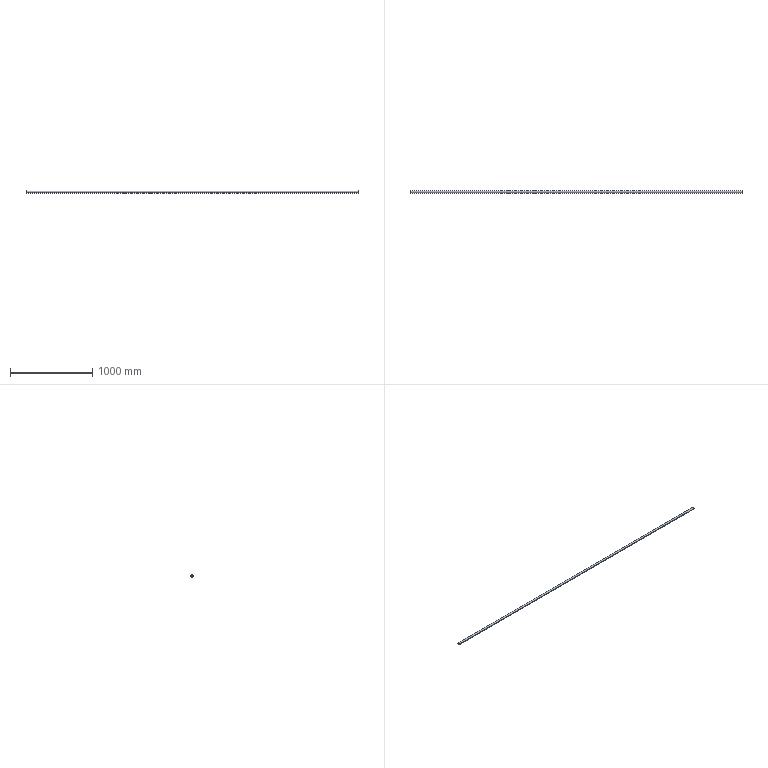Part | STEP file | 电柜护栏1栏杆_Default<As Machined> | 1 solid | 6 faces | box 4025 x 25 x 25 mm | volume 445733 mm3 | cylinder 4 | plane 2 | commonest cylinder face diameters 22 x2 25 x2
STEP:
#1=CARTESIAN_POINT('',(0.,0.,0.));
#2=DIRECTION('',(0.,0.,1.));
#3=DIRECTION('',(1.,0.,0.));
#4=AXIS2_PLACEMENT_3D('',#1,#2,#3);
#5=CARTESIAN_POINT('',(2012.5,12.5,0.));
#6=VERTEX_POINT('',#5);
#7=CARTESIAN_POINT('',(2012.5,-12.5,0.));
#8=VERTEX_POINT('',#7);
#9=CARTESIAN_POINT('',(2012.5,0.,0.));
#10=DIRECTION('',(1.,0.,0.));
#11=DIRECTION('',(0.,1.,0.));
#12=AXIS2_PLACEMENT_3D('',#9,#10,#11);
#13=CIRCLE('',#12,12.5);
#14=CARTESIAN_POINT('',(2012.5,0.,0.));
#15=DIRECTION('',(-1.,0.,0.));
#16=DIRECTION('',(0.,-1.,0.));
#17=AXIS2_PLACEMENT_3D('',#14,#15,#16);
#18=CYLINDRICAL_SURFACE('',#17,12.5);
#19=CARTESIAN_POINT('',(3.142,0.));
#20=DIRECTION('',(-1.,0.));
#21=VECTOR('',#20,1.);
#22=LINE('',#19,#21);
#23=(GEOMETRIC_REPRESENTATION_CONTEXT(2)PARAMETRIC_REPRESENTATION_CONTEXT()REPRESENTATION_CONTEXT('',''));
#24=DEFINITIONAL_REPRESENTATION('',(#22),#23);
#25=PCURVE('',#18,#24);
#26=CARTESIAN_POINT('',(2012.5,0.,0.));
#27=DIRECTION('',(1.,0.,0.));
#28=DIRECTION('',(0.,1.,0.));
#29=AXIS2_PLACEMENT_3D('',#26,#27,#28);
#30=PLANE('',#29);
#31=CARTESIAN_POINT('',(0.,0.));
#32=DIRECTION('',(1.,0.));
#33=AXIS2_PLACEMENT_2D('',#31,#32);
#34=CIRCLE('',#33,12.5);
#35=(GEOMETRIC_REPRESENTATION_CONTEXT(2)PARAMETRIC_REPRESENTATION_CONTEXT()REPRESENTATION_CONTEXT('',''));
#36=DEFINITIONAL_REPRESENTATION('',(#34),#35);
#37=PCURVE('',#30,#36);
#38=SURFACE_CURVE('',#13,(#25,#37),.PCURVE_S1.);
#39=EDGE_CURVE('',#6,#8,#38,.T.);
#40=ORIENTED_EDGE('',*,*,#39,.F.);
#41=CARTESIAN_POINT('',(-2012.5,12.5,0.));
#42=VERTEX_POINT('',#41);
#43=CARTESIAN_POINT('',(2012.5,12.5,0.));
#44=DIRECTION('',(-1.,0.,0.));
#45=VECTOR('',#44,1.);
#46=LINE('',#43,#45);
#47=CARTESIAN_POINT('',(3.142,0.));
#48=DIRECTION('',(0.,1.));
#49=VECTOR('',#48,1.);
#50=LINE('',#47,#49);
#51=(GEOMETRIC_REPRESENTATION_CONTEXT(2)PARAMETRIC_REPRESENTATION_CONTEXT()REPRESENTATION_CONTEXT('',''));
#52=DEFINITIONAL_REPRESENTATION('',(#50),#51);
#53=PCURVE('',#18,#52);
#54=CARTESIAN_POINT('',(2012.5,0.,0.));
#55=DIRECTION('',(-1.,0.,0.));
#56=DIRECTION('',(0.,-1.,0.));
#57=AXIS2_PLACEMENT_3D('',#54,#55,#56);
#58=CYLINDRICAL_SURFACE('',#57,12.5);
#59=CARTESIAN_POINT('',(3.142,0.));
#60=DIRECTION('',(0.,1.));
#61=VECTOR('',#60,1.);
#62=LINE('',#59,#61);
#63=(GEOMETRIC_REPRESENTATION_CONTEXT(2)PARAMETRIC_REPRESENTATION_CONTEXT()REPRESENTATION_CONTEXT('',''));
#64=DEFINITIONAL_REPRESENTATION('',(#62),#63);
#65=PCURVE('',#58,#64);
#66=SURFACE_CURVE('',#46,(#53,#65),.PCURVE_S1.);
#67=EDGE_CURVE('',#6,#42,#66,.T.);
#68=ORIENTED_EDGE('',*,*,#67,.T.);
#69=CARTESIAN_POINT('',(-2012.5,-12.5,0.));
#70=VERTEX_POINT('',#69);
#71=CARTESIAN_POINT('',(-2012.5,0.,0.));
#72=DIRECTION('',(1.,0.,0.));
#73=DIRECTION('',(0.,1.,0.));
#74=AXIS2_PLACEMENT_3D('',#71,#72,#73);
#75=CIRCLE('',#74,12.5);
#76=CARTESIAN_POINT('',(3.142,4025.));
#77=DIRECTION('',(-1.,0.));
#78=VECTOR('',#77,1.);
#79=LINE('',#76,#78);
#80=(GEOMETRIC_REPRESENTATION_CONTEXT(2)PARAMETRIC_REPRESENTATION_CONTEXT()REPRESENTATION_CONTEXT('',''));
#81=DEFINITIONAL_REPRESENTATION('',(#79),#80);
#82=PCURVE('',#18,#81);
#83=CARTESIAN_POINT('',(-2012.5,0.,0.));
#84=DIRECTION('',(1.,0.,0.));
#85=DIRECTION('',(0.,1.,0.));
#86=AXIS2_PLACEMENT_3D('',#83,#84,#85);
#87=PLANE('',#86);
#88=CARTESIAN_POINT('',(0.,0.));
#89=DIRECTION('',(1.,0.));
#90=AXIS2_PLACEMENT_2D('',#88,#89);
#91=CIRCLE('',#90,12.5);
#92=(GEOMETRIC_REPRESENTATION_CONTEXT(2)PARAMETRIC_REPRESENTATION_CONTEXT()REPRESENTATION_CONTEXT('',''));
#93=DEFINITIONAL_REPRESENTATION('',(#91),#92);
#94=PCURVE('',#87,#93);
#95=SURFACE_CURVE('',#75,(#82,#94),.PCURVE_S1.);
#96=EDGE_CURVE('',#42,#70,#95,.T.);
#97=ORIENTED_EDGE('',*,*,#96,.T.);
#98=CARTESIAN_POINT('',(2012.5,-12.5,0.));
#99=DIRECTION('',(-1.,0.,0.));
#100=VECTOR('',#99,1.);
#101=LINE('',#98,#100);
#102=CARTESIAN_POINT('',(0.,0.));
#103=DIRECTION('',(0.,1.));
#104=VECTOR('',#103,1.);
#105=LINE('',#102,#104);
#106=(GEOMETRIC_REPRESENTATION_CONTEXT(2)PARAMETRIC_REPRESENTATION_CONTEXT()REPRESENTATION_CONTEXT('',''));
#107=DEFINITIONAL_REPRESENTATION('',(#105),#106);
#108=PCURVE('',#18,#107);
#109=CARTESIAN_POINT('',(6.283,0.));
#110=DIRECTION('',(0.,1.));
#111=VECTOR('',#110,1.);
#112=LINE('',#109,#111);
#113=(GEOMETRIC_REPRESENTATION_CONTEXT(2)PARAMETRIC_REPRESENTATION_CONTEXT()REPRESENTATION_CONTEXT('',''));
#114=DEFINITIONAL_REPRESENTATION('',(#112),#113);
#115=PCURVE('',#58,#114);
#116=SURFACE_CURVE('',#101,(#108,#115),.PCURVE_S1.);
#117=EDGE_CURVE('',#8,#70,#116,.T.);
#118=ORIENTED_EDGE('',*,*,#117,.F.);
#119=EDGE_LOOP('',(#40,#68,#97,#118));
#120=FACE_BOUND('',#119,.T.);
#121=ADVANCED_FACE('',(#120),#18,.T.);
#122=CARTESIAN_POINT('',(2012.5,-11.,0.));
#123=VERTEX_POINT('',#122);
#124=CARTESIAN_POINT('',(-2012.5,-11.,0.));
#125=VERTEX_POINT('',#124);
#126=CARTESIAN_POINT('',(2012.5,-11.,0.));
#127=DIRECTION('',(-1.,0.,0.));
#128=VECTOR('',#127,1.);
#129=LINE('',#126,#128);
#130=CARTESIAN_POINT('',(2012.5,0.,0.));
#131=DIRECTION('',(-1.,0.,0.));
#132=DIRECTION('',(0.,-1.,0.));
#133=AXIS2_PLACEMENT_3D('',#130,#131,#132);
#134=CYLINDRICAL_SURFACE('',#133,11.);
#135=CARTESIAN_POINT('',(6.283,0.));
#136=DIRECTION('',(0.,1.));
#137=VECTOR('',#136,1.);
#138=LINE('',#135,#137);
#139=(GEOMETRIC_REPRESENTATION_CONTEXT(2)PARAMETRIC_REPRESENTATION_CONTEXT()REPRESENTATION_CONTEXT('',''));
#140=DEFINITIONAL_REPRESENTATION('',(#138),#139);
#141=PCURVE('',#134,#140);
#142=CARTESIAN_POINT('',(2012.5,0.,0.));
#143=DIRECTION('',(-1.,0.,0.));
#144=DIRECTION('',(0.,-1.,0.));
#145=AXIS2_PLACEMENT_3D('',#142,#143,#144);
#146=CYLINDRICAL_SURFACE('',#145,11.);
#147=CARTESIAN_POINT('',(0.,0.));
#148=DIRECTION('',(0.,1.));
#149=VECTOR('',#148,1.);
#150=LINE('',#147,#149);
#151=(GEOMETRIC_REPRESENTATION_CONTEXT(2)PARAMETRIC_REPRESENTATION_CONTEXT()REPRESENTATION_CONTEXT('',''));
#152=DEFINITIONAL_REPRESENTATION('',(#150),#151);
#153=PCURVE('',#146,#152);
#154=SURFACE_CURVE('',#129,(#141,#153),.PCURVE_S1.);
#155=EDGE_CURVE('',#123,#125,#154,.T.);
#156=ORIENTED_EDGE('',*,*,#155,.T.);
#157=CARTESIAN_POINT('',(-2012.5,11.,0.));
#158=VERTEX_POINT('',#157);
#159=CARTESIAN_POINT('',(-2012.5,0.,0.));
#160=DIRECTION('',(1.,0.,0.));
#161=DIRECTION('',(0.,1.,0.));
#162=AXIS2_PLACEMENT_3D('',#159,#160,#161);
#163=CIRCLE('',#162,11.);
#164=CARTESIAN_POINT('',(9.425,4025.));
#165=DIRECTION('',(-1.,0.));
#166=VECTOR('',#165,1.);
#167=LINE('',#164,#166);
#168=(GEOMETRIC_REPRESENTATION_CONTEXT(2)PARAMETRIC_REPRESENTATION_CONTEXT()REPRESENTATION_CONTEXT('',''));
#169=DEFINITIONAL_REPRESENTATION('',(#167),#168);
#170=PCURVE('',#134,#169);
#171=CARTESIAN_POINT('',(0.,0.));
#172=DIRECTION('',(1.,0.));
#173=AXIS2_PLACEMENT_2D('',#171,#172);
#174=CIRCLE('',#173,11.);
#175=(GEOMETRIC_REPRESENTATION_CONTEXT(2)PARAMETRIC_REPRESENTATION_CONTEXT()REPRESENTATION_CONTEXT('',''));
#176=DEFINITIONAL_REPRESENTATION('',(#174),#175);
#177=PCURVE('',#87,#176);
#178=SURFACE_CURVE('',#163,(#170,#177),.PCURVE_S1.);
#179=EDGE_CURVE('',#125,#158,#178,.T.);
#180=ORIENTED_EDGE('',*,*,#179,.T.);
#181=CARTESIAN_POINT('',(2012.5,11.,0.));
#182=VERTEX_POINT('',#181);
#183=CARTESIAN_POINT('',(2012.5,11.,0.));
#184=DIRECTION('',(-1.,0.,0.));
#185=VECTOR('',#184,1.);
#186=LINE('',#183,#185);
#187=CARTESIAN_POINT('',(3.142,0.));
#188=DIRECTION('',(0.,1.));
#189=VECTOR('',#188,1.);
#190=LINE('',#187,#189);
#191=(GEOMETRIC_REPRESENTATION_CONTEXT(2)PARAMETRIC_REPRESENTATION_CONTEXT()REPRESENTATION_CONTEXT('',''));
#192=DEFINITIONAL_REPRESENTATION('',(#190),#191);
#193=PCURVE('',#134,#192);
#194=CARTESIAN_POINT('',(3.142,0.));
#195=DIRECTION('',(0.,1.));
#196=VECTOR('',#195,1.);
#197=LINE('',#194,#196);
#198=(GEOMETRIC_REPRESENTATION_CONTEXT(2)PARAMETRIC_REPRESENTATION_CONTEXT()REPRESENTATION_CONTEXT('',''));
#199=DEFINITIONAL_REPRESENTATION('',(#197),#198);
#200=PCURVE('',#146,#199);
#201=SURFACE_CURVE('',#186,(#193,#200),.PCURVE_S1.);
#202=EDGE_CURVE('',#182,#158,#201,.T.);
#203=ORIENTED_EDGE('',*,*,#202,.F.);
#204=CARTESIAN_POINT('',(2012.5,0.,0.));
#205=DIRECTION('',(1.,0.,0.));
#206=DIRECTION('',(0.,1.,0.));
#207=AXIS2_PLACEMENT_3D('',#204,#205,#206);
#208=CIRCLE('',#207,11.);
#209=CARTESIAN_POINT('',(9.425,0.));
#210=DIRECTION('',(-1.,0.));
#211=VECTOR('',#210,1.);
#212=LINE('',#209,#211);
#213=(GEOMETRIC_REPRESENTATION_CONTEXT(2)PARAMETRIC_REPRESENTATION_CONTEXT()REPRESENTATION_CONTEXT('',''));
#214=DEFINITIONAL_REPRESENTATION('',(#212),#213);
#215=PCURVE('',#134,#214);
#216=CARTESIAN_POINT('',(0.,0.));
#217=DIRECTION('',(1.,0.));
#218=AXIS2_PLACEMENT_2D('',#216,#217);
#219=CIRCLE('',#218,11.);
#220=(GEOMETRIC_REPRESENTATION_CONTEXT(2)PARAMETRIC_REPRESENTATION_CONTEXT()REPRESENTATION_CONTEXT('',''));
#221=DEFINITIONAL_REPRESENTATION('',(#219),#220);
#222=PCURVE('',#30,#221);
#223=SURFACE_CURVE('',#208,(#215,#222),.PCURVE_S1.);
#224=EDGE_CURVE('',#123,#182,#223,.T.);
#225=ORIENTED_EDGE('',*,*,#224,.F.);
#226=EDGE_LOOP('',(#156,#180,#203,#225));
#227=FACE_BOUND('',#226,.F.);
#228=ADVANCED_FACE('',(#227),#134,.F.);
#229=CARTESIAN_POINT('',(-2012.5,0.,0.));
#230=DIRECTION('',(1.,0.,0.));
#231=DIRECTION('',(0.,1.,0.));
#232=AXIS2_PLACEMENT_3D('',#229,#230,#231);
#233=CIRCLE('',#232,11.);
#234=CARTESIAN_POINT('',(3.142,4025.));
#235=DIRECTION('',(-1.,0.));
#236=VECTOR('',#235,1.);
#237=LINE('',#234,#236);
#238=(GEOMETRIC_REPRESENTATION_CONTEXT(2)PARAMETRIC_REPRESENTATION_CONTEXT()REPRESENTATION_CONTEXT('',''));
#239=DEFINITIONAL_REPRESENTATION('',(#237),#238);
#240=PCURVE('',#146,#239);
#241=CARTESIAN_POINT('',(0.,0.));
#242=DIRECTION('',(1.,0.));
#243=AXIS2_PLACEMENT_2D('',#241,#242);
#244=CIRCLE('',#243,11.);
#245=(GEOMETRIC_REPRESENTATION_CONTEXT(2)PARAMETRIC_REPRESENTATION_CONTEXT()REPRESENTATION_CONTEXT('',''));
#246=DEFINITIONAL_REPRESENTATION('',(#244),#245);
#247=PCURVE('',#87,#246);
#248=SURFACE_CURVE('',#233,(#240,#247),.PCURVE_S1.);
#249=EDGE_CURVE('',#158,#125,#248,.T.);
#250=ORIENTED_EDGE('',*,*,#249,.T.);
#251=ORIENTED_EDGE('',*,*,#155,.F.);
#252=CARTESIAN_POINT('',(2012.5,0.,0.));
#253=DIRECTION('',(1.,0.,0.));
#254=DIRECTION('',(0.,1.,0.));
#255=AXIS2_PLACEMENT_3D('',#252,#253,#254);
#256=CIRCLE('',#255,11.);
#257=CARTESIAN_POINT('',(3.142,0.));
#258=DIRECTION('',(-1.,0.));
#259=VECTOR('',#258,1.);
#260=LINE('',#257,#259);
#261=(GEOMETRIC_REPRESENTATION_CONTEXT(2)PARAMETRIC_REPRESENTATION_CONTEXT()REPRESENTATION_CONTEXT('',''));
#262=DEFINITIONAL_REPRESENTATION('',(#260),#261);
#263=PCURVE('',#146,#262);
#264=CARTESIAN_POINT('',(0.,0.));
#265=DIRECTION('',(1.,0.));
#266=AXIS2_PLACEMENT_2D('',#264,#265);
#267=CIRCLE('',#266,11.);
#268=(GEOMETRIC_REPRESENTATION_CONTEXT(2)PARAMETRIC_REPRESENTATION_CONTEXT()REPRESENTATION_CONTEXT('',''));
#269=DEFINITIONAL_REPRESENTATION('',(#267),#268);
#270=PCURVE('',#30,#269);
#271=SURFACE_CURVE('',#256,(#263,#270),.PCURVE_S1.);
#272=EDGE_CURVE('',#182,#123,#271,.T.);
#273=ORIENTED_EDGE('',*,*,#272,.F.);
#274=ORIENTED_EDGE('',*,*,#202,.T.);
#275=EDGE_LOOP('',(#250,#251,#273,#274));
#276=FACE_BOUND('',#275,.F.);
#277=ADVANCED_FACE('',(#276),#146,.F.);
#278=ORIENTED_EDGE('',*,*,#67,.F.);
#279=CARTESIAN_POINT('',(2012.5,0.,0.));
#280=DIRECTION('',(1.,0.,0.));
#281=DIRECTION('',(0.,1.,0.));
#282=AXIS2_PLACEMENT_3D('',#279,#280,#281);
#283=CIRCLE('',#282,12.5);
#284=CARTESIAN_POINT('',(9.425,0.));
#285=DIRECTION('',(-1.,0.));
#286=VECTOR('',#285,1.);
#287=LINE('',#284,#286);
#288=(GEOMETRIC_REPRESENTATION_CONTEXT(2)PARAMETRIC_REPRESENTATION_CONTEXT()REPRESENTATION_CONTEXT('',''));
#289=DEFINITIONAL_REPRESENTATION('',(#287),#288);
#290=PCURVE('',#58,#289);
#291=CARTESIAN_POINT('',(0.,0.));
#292=DIRECTION('',(1.,0.));
#293=AXIS2_PLACEMENT_2D('',#291,#292);
#294=CIRCLE('',#293,12.5);
#295=(GEOMETRIC_REPRESENTATION_CONTEXT(2)PARAMETRIC_REPRESENTATION_CONTEXT()REPRESENTATION_CONTEXT('',''));
#296=DEFINITIONAL_REPRESENTATION('',(#294),#295);
#297=PCURVE('',#30,#296);
#298=SURFACE_CURVE('',#283,(#290,#297),.PCURVE_S1.);
#299=EDGE_CURVE('',#8,#6,#298,.T.);
#300=ORIENTED_EDGE('',*,*,#299,.F.);
#301=ORIENTED_EDGE('',*,*,#117,.T.);
#302=CARTESIAN_POINT('',(-2012.5,0.,0.));
#303=DIRECTION('',(1.,0.,0.));
#304=DIRECTION('',(0.,1.,0.));
#305=AXIS2_PLACEMENT_3D('',#302,#303,#304);
#306=CIRCLE('',#305,12.5);
#307=CARTESIAN_POINT('',(9.425,4025.));
#308=DIRECTION('',(-1.,0.));
#309=VECTOR('',#308,1.);
#310=LINE('',#307,#309);
#311=(GEOMETRIC_REPRESENTATION_CONTEXT(2)PARAMETRIC_REPRESENTATION_CONTEXT()REPRESENTATION_CONTEXT('',''));
#312=DEFINITIONAL_REPRESENTATION('',(#310),#311);
#313=PCURVE('',#58,#312);
#314=CARTESIAN_POINT('',(0.,0.));
#315=DIRECTION('',(1.,0.));
#316=AXIS2_PLACEMENT_2D('',#314,#315);
#317=CIRCLE('',#316,12.5);
#318=(GEOMETRIC_REPRESENTATION_CONTEXT(2)PARAMETRIC_REPRESENTATION_CONTEXT()REPRESENTATION_CONTEXT('',''));
#319=DEFINITIONAL_REPRESENTATION('',(#317),#318);
#320=PCURVE('',#87,#319);
#321=SURFACE_CURVE('',#306,(#313,#320),.PCURVE_S1.);
#322=EDGE_CURVE('',#70,#42,#321,.T.);
#323=ORIENTED_EDGE('',*,*,#322,.T.);
#324=EDGE_LOOP('',(#278,#300,#301,#323));
#325=FACE_BOUND('',#324,.T.);
#326=ADVANCED_FACE('',(#325),#58,.T.);
#327=ORIENTED_EDGE('',*,*,#224,.F.);
#328=ORIENTED_EDGE('',*,*,#272,.F.);
#329=EDGE_LOOP('',(#327,#328));
#330=FACE_BOUND('',#329,.T.);
#331=ORIENTED_EDGE('',*,*,#299,.T.);
#332=ORIENTED_EDGE('',*,*,#39,.T.);
#333=EDGE_LOOP('',(#331,#332));
#334=FACE_BOUND('',#333,.T.);
#335=ADVANCED_FACE('',(#330,#334),#30,.T.);
#336=ORIENTED_EDGE('',*,*,#179,.T.);
#337=ORIENTED_EDGE('',*,*,#249,.T.);
#338=EDGE_LOOP('',(#336,#337));
#339=FACE_BOUND('',#338,.T.);
#340=ORIENTED_EDGE('',*,*,#322,.F.);
#341=ORIENTED_EDGE('',*,*,#96,.F.);
#342=EDGE_LOOP('',(#340,#341));
#343=FACE_BOUND('',#342,.T.);
#344=ADVANCED_FACE('',(#339,#343),#87,.F.);
#345=CLOSED_SHELL('',(#121,#228,#277,#326,#335,#344));
#346=MANIFOLD_SOLID_BREP('',#345);
#347=(LENGTH_UNIT()NAMED_UNIT(*)SI_UNIT(.MILLI.,.METRE.));
#348=UNCERTAINTY_MEASURE_WITH_UNIT(LENGTH_MEASURE(0.0000001),#347,'','');
#349=(NAMED_UNIT(*)PLANE_ANGLE_UNIT()SI_UNIT($,.RADIAN.));
#350=(NAMED_UNIT(*)SI_UNIT($,.STERADIAN.)SOLID_ANGLE_UNIT());
#351=(GEOMETRIC_REPRESENTATION_CONTEXT(3)GLOBAL_UNCERTAINTY_ASSIGNED_CONTEXT((#348))GLOBAL_UNIT_ASSIGNED_CONTEXT((#347,#349,#350))REPRESENTATION_CONTEXT('',''));
#352=ADVANCED_BREP_SHAPE_REPRESENTATION('',(#4,#346),#351);